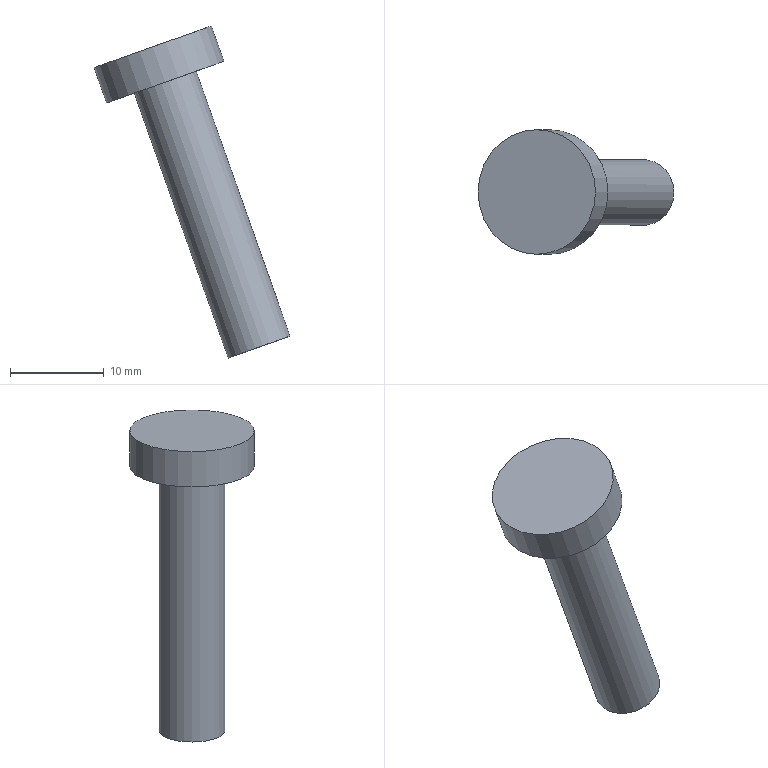Part | STEP file | SLIDE1-INSERT3_id690_x_t | 1 solid | 5 faces | box 20.917 x 13.3 x 35.438 mm | volume 1710 mm3 | plane 3 | cylinder 2 | commonest cylinder face diameters 7 x1 13.3 x1
STEP:
#1=CARTESIAN_POINT('',(-9.969,0.,-49.977));
#2=VERTEX_POINT('',#1);
#3=CARTESIAN_POINT('',(-3.7,0.,-47.757));
#4=DIRECTION('',(0.3338,0.,-0.9426));
#5=DIRECTION('',(-0.9426,0.,-0.3338));
#6=AXIS2_PLACEMENT_3D('',#3,#4,#5);
#7=CIRCLE('',#6,6.65);
#8=EDGE_CURVE('',#2,#2,#7,.T.);
#9=ORIENTED_EDGE('',*,*,#8,.F.);
#10=EDGE_LOOP('',(#9));
#11=FACE_OUTER_BOUND('',#10,.T.);
#12=CARTESIAN_POINT('',(-3.7,0.,-47.757));
#13=DIRECTION('',(0.3338,0.,-0.9426));
#14=DIRECTION('',(-0.9426,0.,-0.3338));
#15=AXIS2_PLACEMENT_3D('',#12,#13,#14);
#16=PLANE('',#15);
#17=ADVANCED_FACE('',(#11),#16,.F.);
#18=ORIENTED_EDGE('',*,*,#8,.T.);
#19=EDGE_LOOP('',(#18));
#20=FACE_BOUND('',#19,.T.);
#21=CARTESIAN_POINT('',(-8.634,0.,-53.747));
#22=VERTEX_POINT('',#21);
#23=CARTESIAN_POINT('',(-2.365,0.,-51.528));
#24=DIRECTION('',(0.3338,0.,-0.9426));
#25=DIRECTION('',(-0.9426,0.,-0.3338));
#26=AXIS2_PLACEMENT_3D('',#23,#24,#25);
#27=CIRCLE('',#26,6.65);
#28=EDGE_CURVE('',#22,#22,#27,.T.);
#29=ORIENTED_EDGE('',*,*,#28,.F.);
#30=EDGE_LOOP('',(#29));
#31=FACE_BOUND('',#30,.T.);
#32=CARTESIAN_POINT('',(-4.268,0.,-46.154));
#33=DIRECTION('',(0.3338,0.,-0.9426));
#34=DIRECTION('',(-0.9426,0.,-0.3338));
#35=AXIS2_PLACEMENT_3D('',#32,#33,#34);
#36=CYLINDRICAL_SURFACE('',#35,6.65);
#37=ADVANCED_FACE('',(#20,#31),#36,.T.);
#38=CARTESIAN_POINT('',(4.35,0.,-80.975));
#39=VERTEX_POINT('',#38);
#40=CARTESIAN_POINT('',(7.649,0.,-79.807));
#41=DIRECTION('',(-0.3338,0.,0.9426));
#42=DIRECTION('',(-0.9426,0.,-0.3338));
#43=AXIS2_PLACEMENT_3D('',#40,#41,#42);
#44=CIRCLE('',#43,3.5);
#45=EDGE_CURVE('',#39,#39,#44,.T.);
#46=ORIENTED_EDGE('',*,*,#45,.F.);
#47=EDGE_LOOP('',(#46));
#48=FACE_OUTER_BOUND('',#47,.T.);
#49=CARTESIAN_POINT('',(7.649,0.,-79.807));
#50=DIRECTION('',(0.3338,0.,-0.9426));
#51=DIRECTION('',(-0.9426,0.,-0.3338));
#52=AXIS2_PLACEMENT_3D('',#49,#50,#51);
#53=PLANE('',#52);
#54=ADVANCED_FACE('',(#48),#53,.T.);
#55=CARTESIAN_POINT('',(-5.664,0.,-52.696));
#56=VERTEX_POINT('',#55);
#57=CARTESIAN_POINT('',(-2.365,0.,-51.528));
#58=DIRECTION('',(0.3338,0.,-0.9426));
#59=DIRECTION('',(-0.9426,0.,-0.3338));
#60=AXIS2_PLACEMENT_3D('',#57,#58,#59);
#61=CIRCLE('',#60,3.5);
#62=EDGE_CURVE('',#56,#56,#61,.T.);
#63=ORIENTED_EDGE('',*,*,#62,.F.);
#64=EDGE_LOOP('',(#63));
#65=FACE_BOUND('',#64,.T.);
#66=ORIENTED_EDGE('',*,*,#28,.T.);
#67=EDGE_LOOP('',(#66));
#68=FACE_BOUND('',#67,.T.);
#69=CARTESIAN_POINT('',(-2.365,0.,-51.528));
#70=DIRECTION('',(0.3338,0.,-0.9426));
#71=DIRECTION('',(-0.9426,0.,-0.3338));
#72=AXIS2_PLACEMENT_3D('',#69,#70,#71);
#73=PLANE('',#72);
#74=ADVANCED_FACE('',(#65,#68),#73,.T.);
#75=ORIENTED_EDGE('',*,*,#62,.T.);
#76=EDGE_LOOP('',(#75));
#77=FACE_BOUND('',#76,.T.);
#78=ORIENTED_EDGE('',*,*,#45,.T.);
#79=EDGE_LOOP('',(#78));
#80=FACE_BOUND('',#79,.T.);
#81=CARTESIAN_POINT('',(-4.268,0.,-46.154));
#82=DIRECTION('',(0.3338,0.,-0.9426));
#83=DIRECTION('',(-0.9426,0.,-0.3338));
#84=AXIS2_PLACEMENT_3D('',#81,#82,#83);
#85=CYLINDRICAL_SURFACE('',#84,3.5);
#86=ADVANCED_FACE('',(#77,#80),#85,.T.);
#87=CLOSED_SHELL('',(#17,#37,#54,#74,#86));
#88=MANIFOLD_SOLID_BREP('',#87);
#89=(LENGTH_UNIT()NAMED_UNIT(*)SI_UNIT(.MILLI.,.METRE.));
#90=UNCERTAINTY_MEASURE_WITH_UNIT(LENGTH_MEASURE(0.00002),#89,'','');
#91=(NAMED_UNIT(*)PLANE_ANGLE_UNIT()SI_UNIT($,.RADIAN.));
#92=PLANE_ANGLE_MEASURE_WITH_UNIT(PLANE_ANGLE_MEASURE(0.01745),#91);
#93=DIMENSIONAL_EXPONENTS(0.,0.,0.,0.,0.,0.,0.);
#94=(CONVERSION_BASED_UNIT('DEGREE',#92)NAMED_UNIT(#93)PLANE_ANGLE_UNIT());
#95=(NAMED_UNIT(*)SI_UNIT($,.STERADIAN.)SOLID_ANGLE_UNIT());
#96=(GEOMETRIC_REPRESENTATION_CONTEXT(3)GLOBAL_UNCERTAINTY_ASSIGNED_CONTEXT((#90))GLOBAL_UNIT_ASSIGNED_CONTEXT((#89,#94,#95))REPRESENTATION_CONTEXT('',''));
#97=ADVANCED_BREP_SHAPE_REPRESENTATION('',(#88),#96);